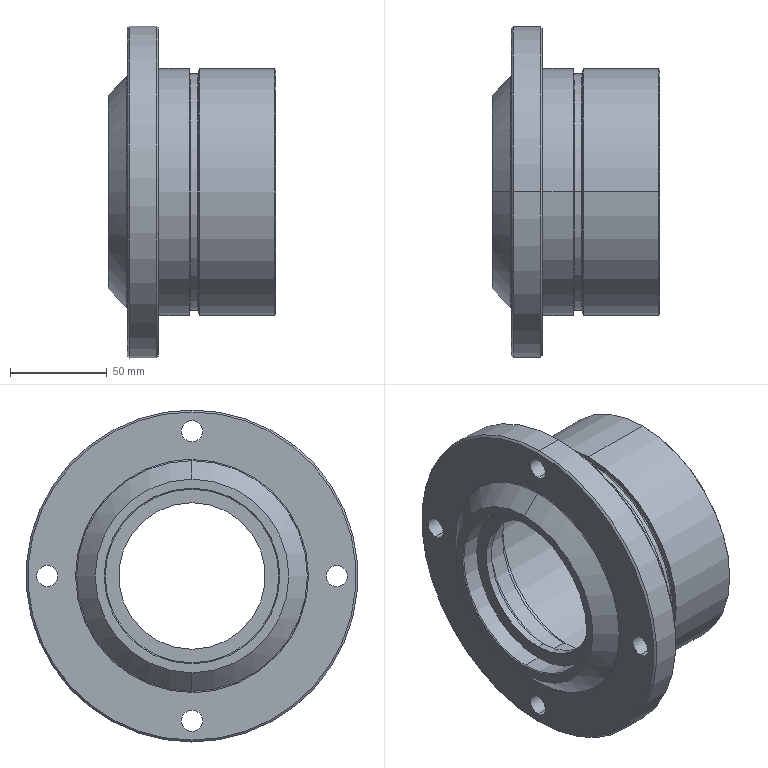Part | SolidWorks | features BaseBody 1 | 1 solid | 74 faces | box 86.84 x 172 x 172 mm | volume 518697 mm3 | cylinder 30 | spline 18 | cone 16 | plane 10 | commonest cylinder face diameters 11 x8 90 x4 110 x4 128 x4 76 x2 100 x2